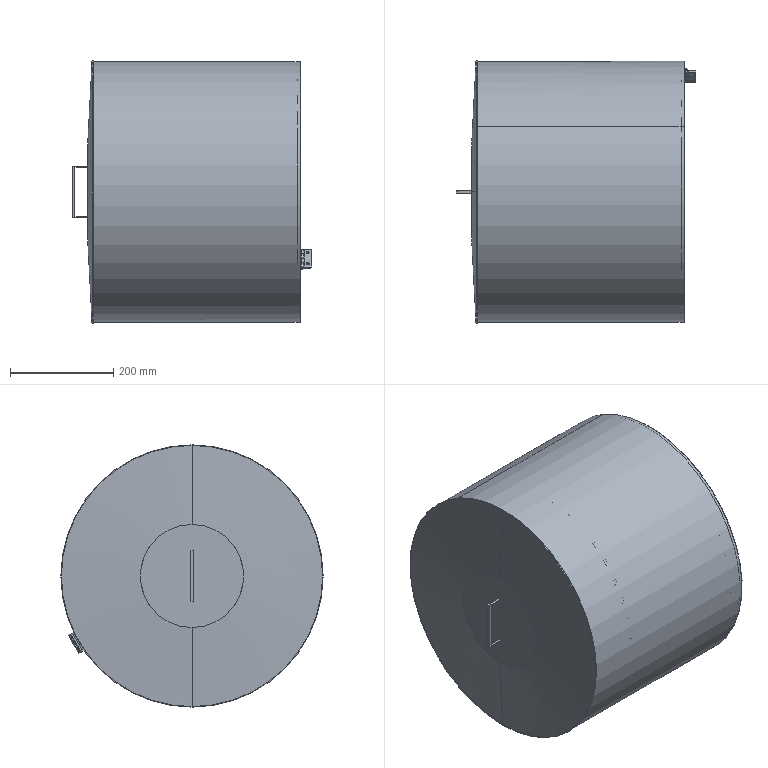Part | SolidWorks | features ReferencePattern 3, LocalCirPattern 1 | 11 solids | 204 faces | box 463.5 x 508 x 508 mm | volume 4178464 mm3 | cylinder 104 | plane 88 | cone 12 | commonest cylinder face diameters 6 x24 150 x16 154 x16 4 x10 500 x8 5 x4